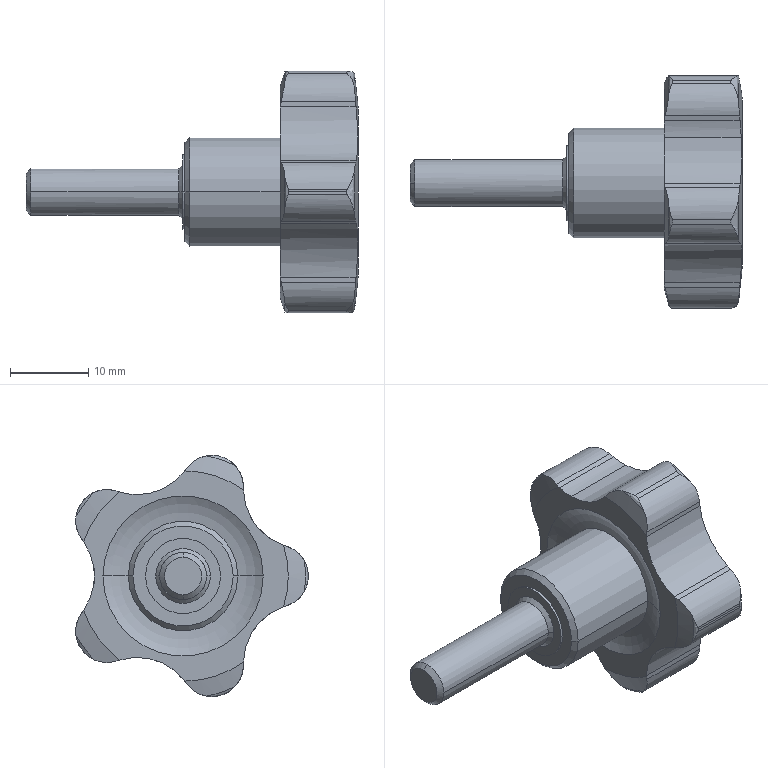Part | SolidWorks | features BaseBody 1 | 1 solid | 73 faces | box 42.423 x 29.716 x 30.844 mm | volume 7689 mm3 | cylinder 30 | cone 15 | plane 14 | spline 10 | torus 4 | commonest cylinder face diameters 8 x12 15 x6 32 x6 6 x2 9.6 x2 14 x2